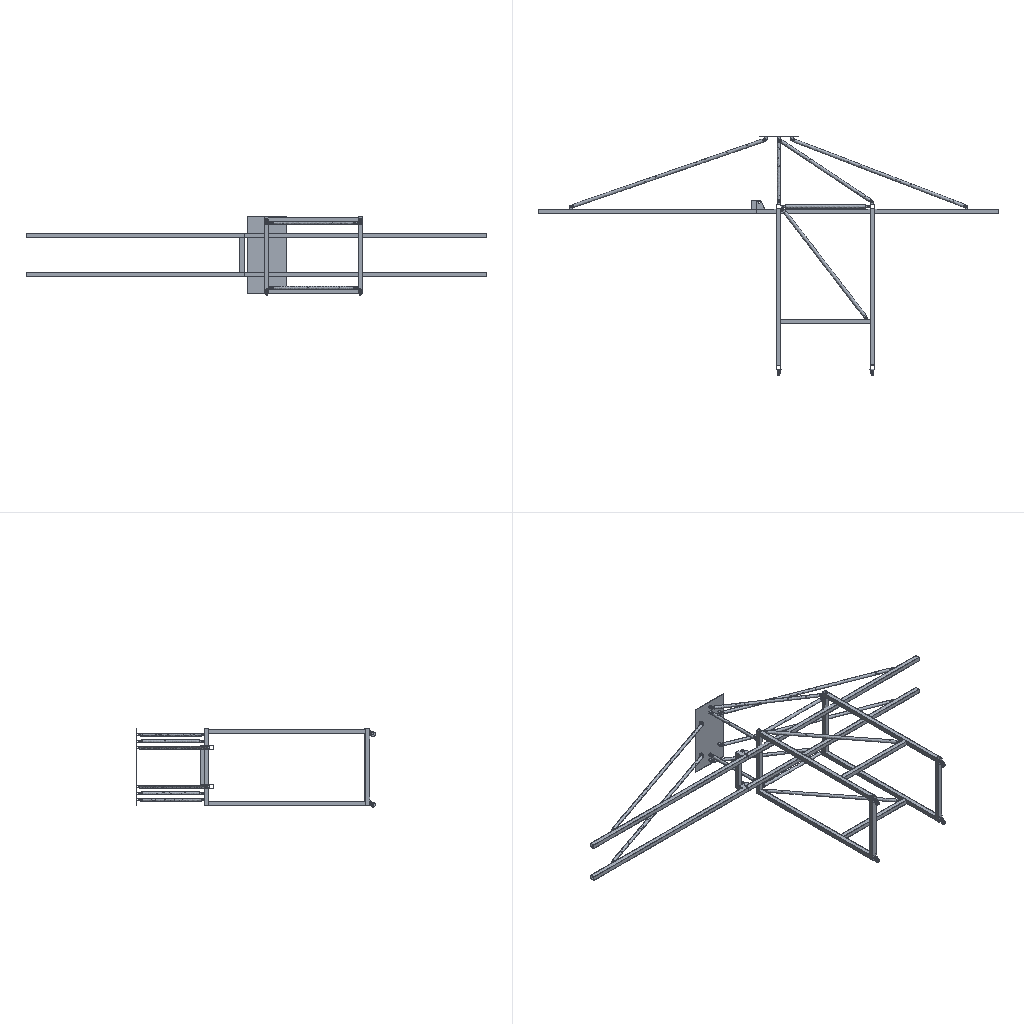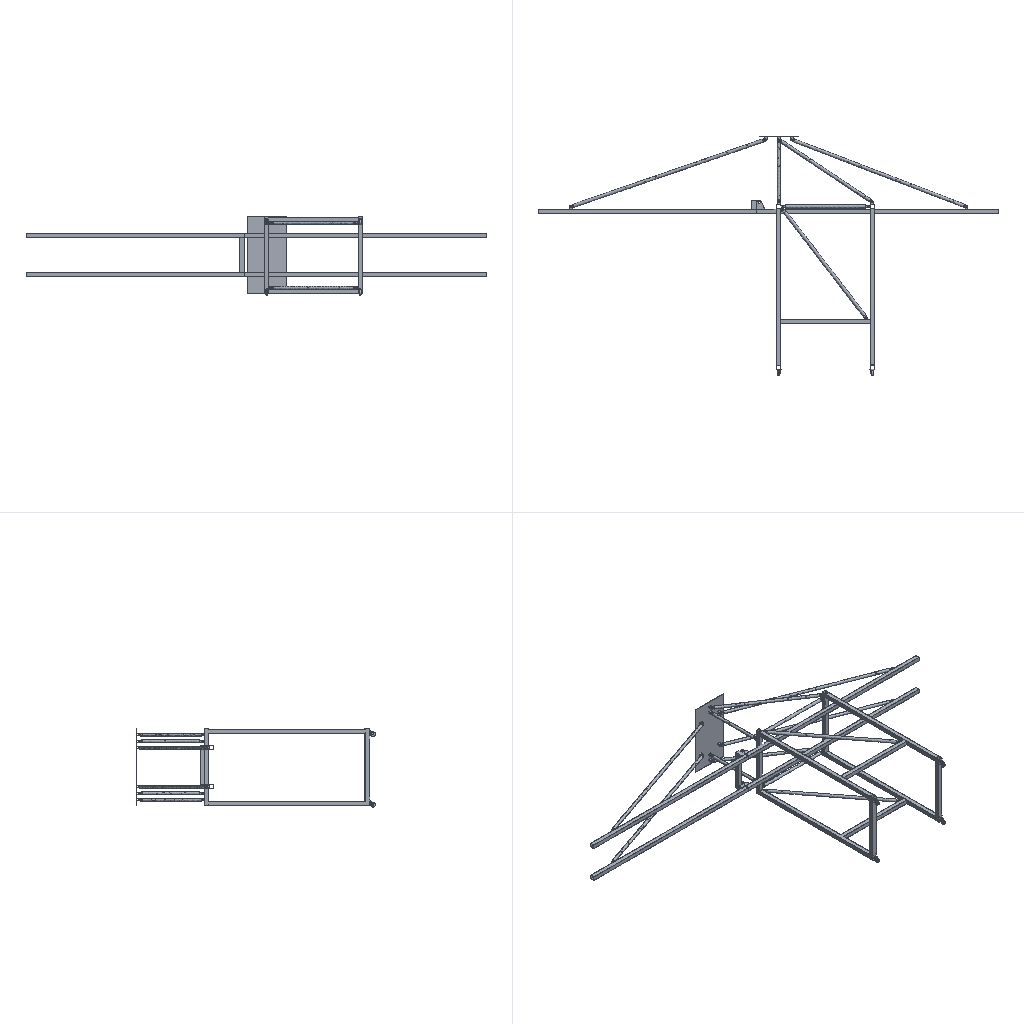Simulation study | ansys workbench
Set-up summary:
category,name,step,type,value,unit,region
solver,ansys_workbench
units,mm-N-s-tonne (MPa),,stated,"/units,MPA"
analysis,deck-1/LS1,,static
load_step,deck-1/LS1,deck-1/LS1,static,nsubst=1; time=1
analysis,deck-2/LS1,,static
load_step,deck-2/LS1,deck-2/LS1,static,nsubst=1; time=1
mesh,deck-1.dat,,nodes,355068
mesh,deck-1.dat,,elements,248214
element_type,SOLID187,,,132266,,deck-1.dat
element_type,SHELL181,,,96130,,deck-1.dat
element_type,SURF154,,,9834,,deck-1.dat
element_type,CONTA174,,,4930,,deck-1.dat
element_type,TARGE170,,,4392,,deck-1.dat
element_type,SOLID186,,,662,,deck-1.dat
mesh,deck-2.dat,,nodes,355072
mesh,deck-2.dat,,elements,248598
element_type,SOLID187,,,132266,,deck-2.dat
element_type,SHELL181,,,96130,,deck-2.dat
element_type,SURF154,,,9834,,deck-2.dat
element_type,CONTA174,,,5314,,deck-2.dat
element_type,TARGE170,,,4392,,deck-2.dat
element_type,SOLID186,,,662,,deck-2.dat
material,Structural Steel,,E,200000,tonne s^-2 mm^-1
material,Structural Steel,,nu,0.3
material,Structural Steel,,density,7.85e-09,tonne mm^-3
material,Structural Steel,,conductivity,60.5,tonne mm s^-3 C^-1
material,Structural Steel,,specific_heat,4.34e+08,mm^2 s^-2 C^-1
material,Structural Steel,,cte,1.2e-05,C^-1
material,Structural Steel,,permeability,10000
material,Structural Steel,,resistivity,0.00017,ohm mm
load,Define Force Using Surface Effect Elements,deck-1/LS1,surface-effect pres face 2,-0.01085,,SURF154 #251
load,Define Force Using Surface Effect Elements,deck-2/LS1,surface-effect pres face 2,-0.01085,,SURF154 #259
bc,Fixed Supports,deck-1/model,fixed,[dofs=ALL],,_FIXEDSU
bc,,deck-2/LS1,fixed,"[dofs=UX,UY,UZ n=8]",,node list
contact,Contact Region,,bonded (always),element=CONTA174
contact,Contact Region 2,,bonded (always),element=CONTA174
contact,Contact Region 3,,bonded (always),element=CONTA174
contact,Contact Region 4,,bonded (always),element=CONTA174
contact,Contact Region,,bonded (always),element=CONTA174
contact,Contact Region 2,,bonded (always),element=CONTA174
contact,Contact Region 3,,bonded (always),element=CONTA174
contact,Contact Region 4,,bonded (always),element=CONTA174
contact,Contact Region 5,,bonded (always),element=CONTA174
contact,Contact Region 6,,bonded (always),element=CONTA174
contact,Contact Region 7,,bonded (always),element=CONTA174
contact,Contact Region 8,,bonded (always),element=CONTA174
contact,Contact Region,,bonded (always),element=CONTA174
contact,Contact Region 2,,bonded (always),element=CONTA174
contact,Contact Region,,bonded (always),element=CONTA174
contact,Contact Region 2,,bonded (always),element=CONTA174
contact,Contact Region,,bonded (always),element=CONTA174
contact,Contact Region 2,,bonded (always),element=CONTA174
contact,Contact Region 3,,bonded (always),element=CONTA174
contact,Contact Region 4,,bonded (always),element=CONTA174
contact,contact 21,,bonded (always),element=CONTA174
contact,contact 22,,bonded (always),element=CONTA175
contact,contact 23,,bonded (always),element=CONTA174
contact,contact 24,,bonded (always),element=CONTA175
contact,contact 25,,bonded (always),element=CONTA174
contact,contact 26,,bonded (always),element=CONTA175
contact,contact 27,,bonded (always),element=CONTA174
contact,contact 28,,bonded (always),element=CONTA175
contact,contact 29,,bonded (always),element=CONTA174
contact,contact 30,,bonded (always),element=CONTA175
contact,contact 31,,bonded (always),element=CONTA174
contact,contact 32,,bonded (always),element=CONTA175
contact,contact 33,,bonded (always),element=CONTA174
contact,contact 34,,bonded (always),element=CONTA175
contact,contact 35,,bonded (always),element=CONTA174
contact,contact 36,,bonded (always),element=CONTA175
contact,contact 37,,bonded (always),element=CONTA174
contact,contact 38,,bonded (always),element=CONTA175
contact,contact 39,,bonded (always),element=CONTA174
contact,contact 40,,bonded (always),element=CONTA175
contact,contact 41,,bonded (always),element=CONTA174
contact,contact 42,,bonded (always),element=CONTA175
contact,contact 43,,bonded (always),element=CONTA174
contact,contact 44,,bonded (always),element=CONTA175
contact,contact 45,,bonded (always),element=CONTA174
contact,contact 46,,bonded (always),element=CONTA175
contact,contact 47,,bonded (always),element=CONTA174
contact,contact 48,,bonded (always),element=CONTA175
contact,contact 49,,bonded (always),element=CONTA174
contact,contact 50,,bonded (always),element=CONTA175
contact,contact 51,,bonded (always),element=CONTA174
contact,contact 52,,bonded (always),element=CONTA175
contact,contact 53,,bonded (always),element=CONTA174
contact,contact 54,,bonded (always),element=CONTA175
contact,contact 55,,bonded (always),element=CONTA174
contact,contact 56,,bonded (always),element=CONTA175
contact,contact 57,,bonded (always),element=CONTA174
contact,contact 58,,bonded (always),element=CONTA174
contact,contact 59,,bonded (always),element=CONTA174
contact,contact 60,,bonded (always),element=CONTA174
contact,contact 61,,bonded (always),element=CONTA174
contact,contact 62,,bonded (always),element=CONTA174
contact,contact 63,,bonded (always),element=CONTA174
contact,contact 64,,bonded (always),element=CONTA174
contact,contact 65,,bonded (always),element=CONTA174
contact,contact 66,,bonded (always),element=CONTA174
contact,contact 67,,bonded (always),element=CONTA174
contact,contact 68,,bonded (always),element=CONTA174
contact,contact 69,,bonded (always),element=CONTA174
contact,contact 70,,bonded (always),element=CONTA174
contact,contact 71,,bonded (always),element=CONTA174
contact,contact 72,,bonded (always),element=CONTA174
contact,Contact Region,,bonded (always),element=CONTA174
contact,Contact Region 2,,bonded (always),element=CONTA174
contact,Contact Region 3,,bonded (always),element=CONTA174
contact,Contact Region 4,,bonded (always),element=CONTA174
contact,Contact Region,,bonded (always),element=CONTA174
contact,Contact Region 2,,bonded (always),element=CONTA174
contact,Contact Region 3,,bonded (always),element=CONTA174
contact,Contact Region 4,,bonded (always),element=CONTA174
contact,Contact Region 5,,bonded (always),element=CONTA174
contact,Contact Region 6,,bonded (always),element=CONTA174
contact,Contact Region 7,,bonded (always),element=CONTA174
contact,Contact Region 8,,bonded (always),element=CONTA174
contact,Contact Region,,bonded (always),element=CONTA174
contact,Contact Region 2,,bonded (always),element=CONTA174
contact,Contact Region,,bonded (always),element=CONTA174
contact,Contact Region 2,,bonded (always),element=CONTA174
contact,Contact Region,,bonded (always),element=CONTA174
contact,Contact Region 2,,bonded (always),element=CONTA174
contact,Contact Region 3,,bonded (always),element=CONTA174
contact,Contact Region 4,,bonded (always),element=CONTA174
contact,contact 21,,bonded (always),element=CONTA174
contact,contact 22,,bonded (always),element=CONTA175
contact,contact 23,,bonded (always),element=CONTA174
contact,contact 24,,bonded (always),element=CONTA175
contact,contact 25,,bonded (always),element=CONTA174
contact,contact 26,,bonded (always),element=CONTA175
contact,contact 27,,bonded (always),element=CONTA174
contact,contact 28,,bonded (always),element=CONTA175
contact,contact 29,,bonded (always),element=CONTA174
contact,contact 30,,bonded (always),element=CONTA175
contact,contact 31,,bonded (always),element=CONTA174
contact,contact 32,,bonded (always),element=CONTA175
contact,contact 33,,bonded (always),element=CONTA174
contact,contact 34,,bonded (always),element=CONTA175
contact,contact 35,,bonded (always),element=CONTA174
contact,contact 36,,bonded (always),element=CONTA175
contact,contact 37,,bonded (always),element=CONTA174
contact,contact 38,,bonded (always),element=CONTA175
contact,contact 39,,bonded (always),element=CONTA174
contact,contact 40,,bonded (always),element=CONTA175
contact,contact 41,,bonded (always),element=CONTA174
contact,contact 42,,bonded (always),element=CONTA175
contact,contact 43,,bonded (always),element=CONTA174
contact,contact 44,,bonded (always),element=CONTA175
contact,contact 45,,bonded (always),element=CONTA174
contact,contact 46,,bonded (always),element=CONTA175
contact,contact 47,,bonded (always),element=CONTA174
contact,contact 48,,bonded (always),element=CONTA175
contact,contact 49,,bonded (always),element=CONTA174
contact,contact 50,,bonded (always),element=CONTA175
contact,contact 51,,bonded (always),element=CONTA174
contact,contact 52,,bonded (always),element=CONTA175
contact,contact 53,,bonded (always),element=CONTA174
contact,contact 54,,bonded (always),element=CONTA175
contact,contact 55,,bonded (always),element=CONTA174
contact,contact 56,,bonded (always),element=CONTA175
contact,contact 57,,bonded (always),element=CONTA174
contact,contact 58,,bonded (always),element=CONTA174
contact,contact 59,,bonded (always),element=CONTA174
contact,contact 60,,bonded (always),element=CONTA174
contact,contact 61,,bonded (always),element=CONTA174
contact,contact 62,,bonded (always),element=CONTA174
contact,contact 63,,bonded (always),element=CONTA174
contact,contact 64,,bonded (always),element=CONTA174
contact,contact 65,,bonded (always),element=CONTA174
contact,contact 66,,bonded (always),element=CONTA174
contact,contact 67,,bonded (always),element=CONTA174
contact,contact 68,,bonded (always),element=CONTA174
contact,contact 69,,bonded (always),element=CONTA174
contact,contact 70,,bonded (always),element=CONTA174
contact,contact 71,,bonded (always),element=CONTA174
contact,contact 72,,bonded (always),element=CONTA174
contact,contact 73,,bonded (always),element=CONTA174
contact,contact 74,,bonded (always),element=CONTA174
contact,contact 75,,bonded (always),element=CONTA174
contact,contact 76,,bonded (always),element=CONTA174
named_set,_FIXEDSU,,node,960
named_set,REMOTEDISPALL,,node,4
Results summary:
result,analyses[0].index,,,1
result,analyses[0].system,,,SYS
result,analyses[0].deck,,,deck-1.dat
result,analyses[0].solve_status,,,completed
result,analyses[0].analysis_type,,,static
result,analyses[0].physics,,,mechanical
result,analyses[0].unit_system,,,"NMM: mm, ton, N, s, mV, mA, degC"
result,analyses[0].n_sets,,,1
result,analyses[0].load_steps[0].set,set=1,,1
result,analyses[0].load_steps[0].time_or_freq,set=1,,1
result,analyses[0].load_steps[0].max_displacement_magnitude,set=1,,4683.72
result,analyses[0].load_steps[0].max_von_mises_nodal,set=1,,1560.47
result,analyses[0].load_steps[0].reaction_force_sum_xyz[1],set=1,,8.33798e-06
result,analyses[0].load_steps[0].reaction_force_sum_xyz[2],set=1,,10000
result,analyses[0].load_steps[0].reaction_force_sum_xyz[3],set=1,,3.33909e-06
result,analyses[1].index,,,2
result,analyses[1].system,,,SYS-1
result,analyses[1].deck,,,deck-2.dat
result,analyses[1].solve_status,,,completed
result,analyses[1].analysis_type,,,static
result,analyses[1].physics,,,mechanical
result,analyses[1].unit_system,,,"NMM: mm, ton, N, s, mV, mA, degC"
result,analyses[1].n_sets,,,1
result,analyses[1].load_steps[0].set,set=1,,1
result,analyses[1].load_steps[0].time_or_freq,set=1,,1
result,analyses[1].load_steps[0].max_displacement_magnitude,set=1,,4685.11
result,analyses[1].load_steps[0].max_von_mises_nodal,set=1,,7129.18
result,analyses[1].load_steps[0].reaction_force_sum_xyz[1],set=1,,3.14145e-05
result,analyses[1].load_steps[0].reaction_force_sum_xyz[2],set=1,,10000
result,analyses[1].load_steps[0].reaction_force_sum_xyz[3],set=1,,0.0001571
result,geometry_export[0][0],,,.step
result,geometry_export[0][1],,,ok
result,geometry_export[0][2],,,134